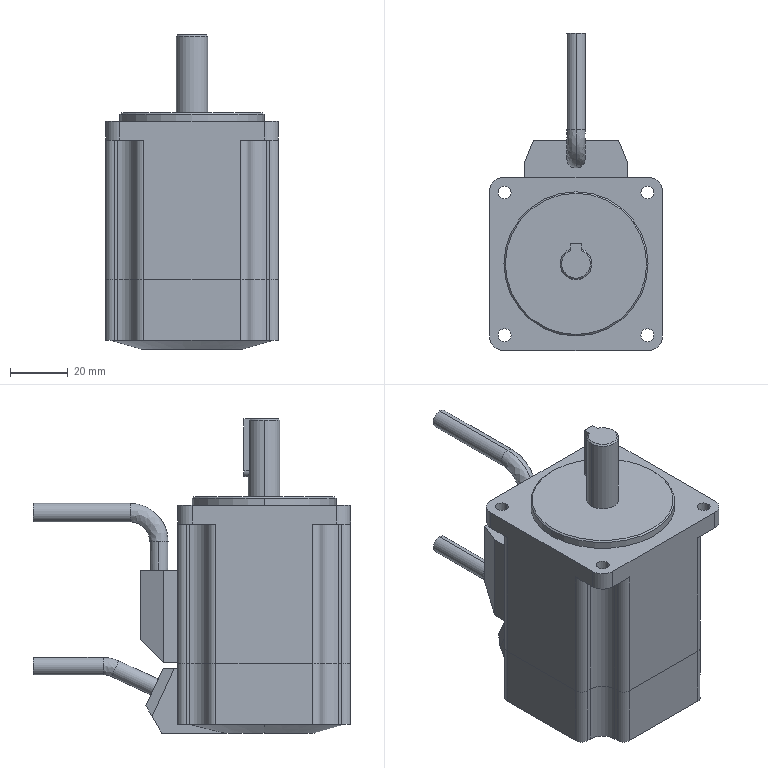Part | STEP file | Servo motor MSMD022P1U_Panasonic_default | 2 solids | 118 faces | box 60 x 110 x 109 mm | volume 279096 mm3 | plane 58 | cylinder 50 | cone 6 | spline 4 | commonest cylinder face diameters 6 x20 4.5 x8 12 x8 6.4 x4 10 x4 4 x2